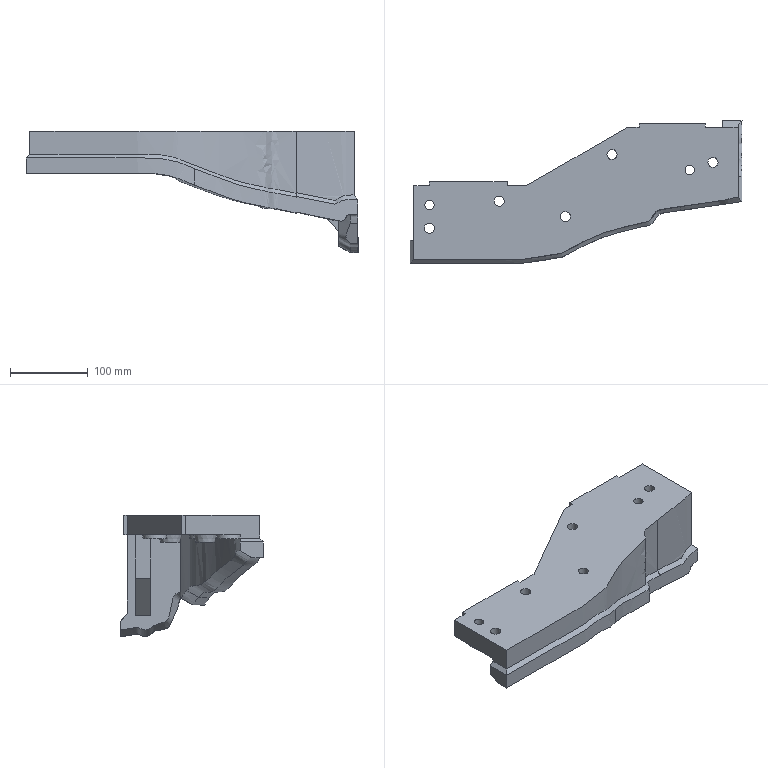Part | NX | features solid 2 | 1 solid | 71 faces | box 427.317 x 183.936 x 156.518 mm | volume 1900966 mm3 | plane 39 | spline 15 | cylinder 15 | cone 2 | commonest cylinder face diameters 13 x7 30 x6 12 x2